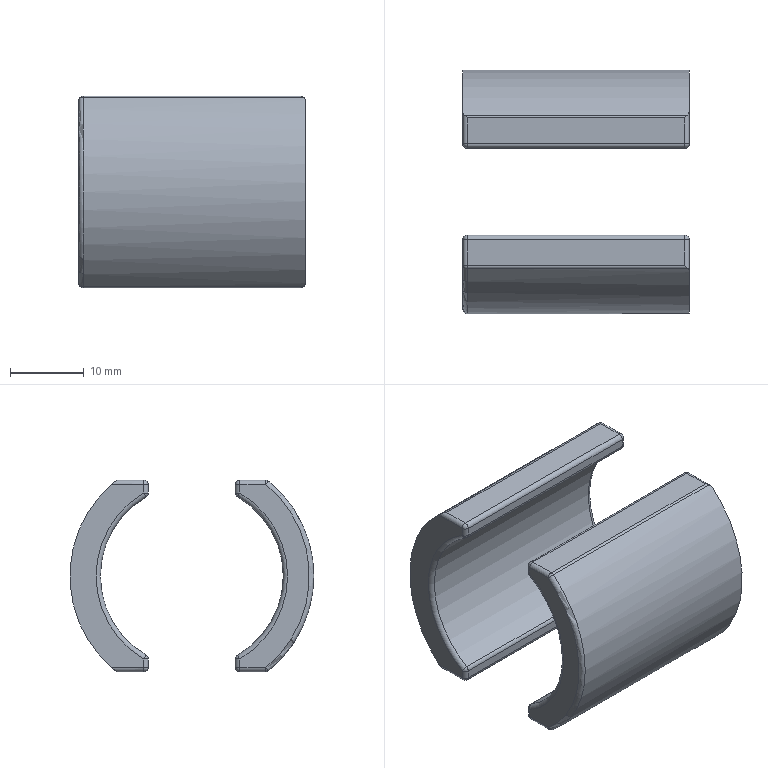Part | SolidWorks | features BaseBody 2 | 2 solids | 67 faces | box 30.643 x 33 x 25.929 mm | volume 7646 mm3 | cylinder 32 | sphere 18 | plane 12 | torus 5 | commonest cylinder face diameters 1.179 x28 24.75 x2 33 x2